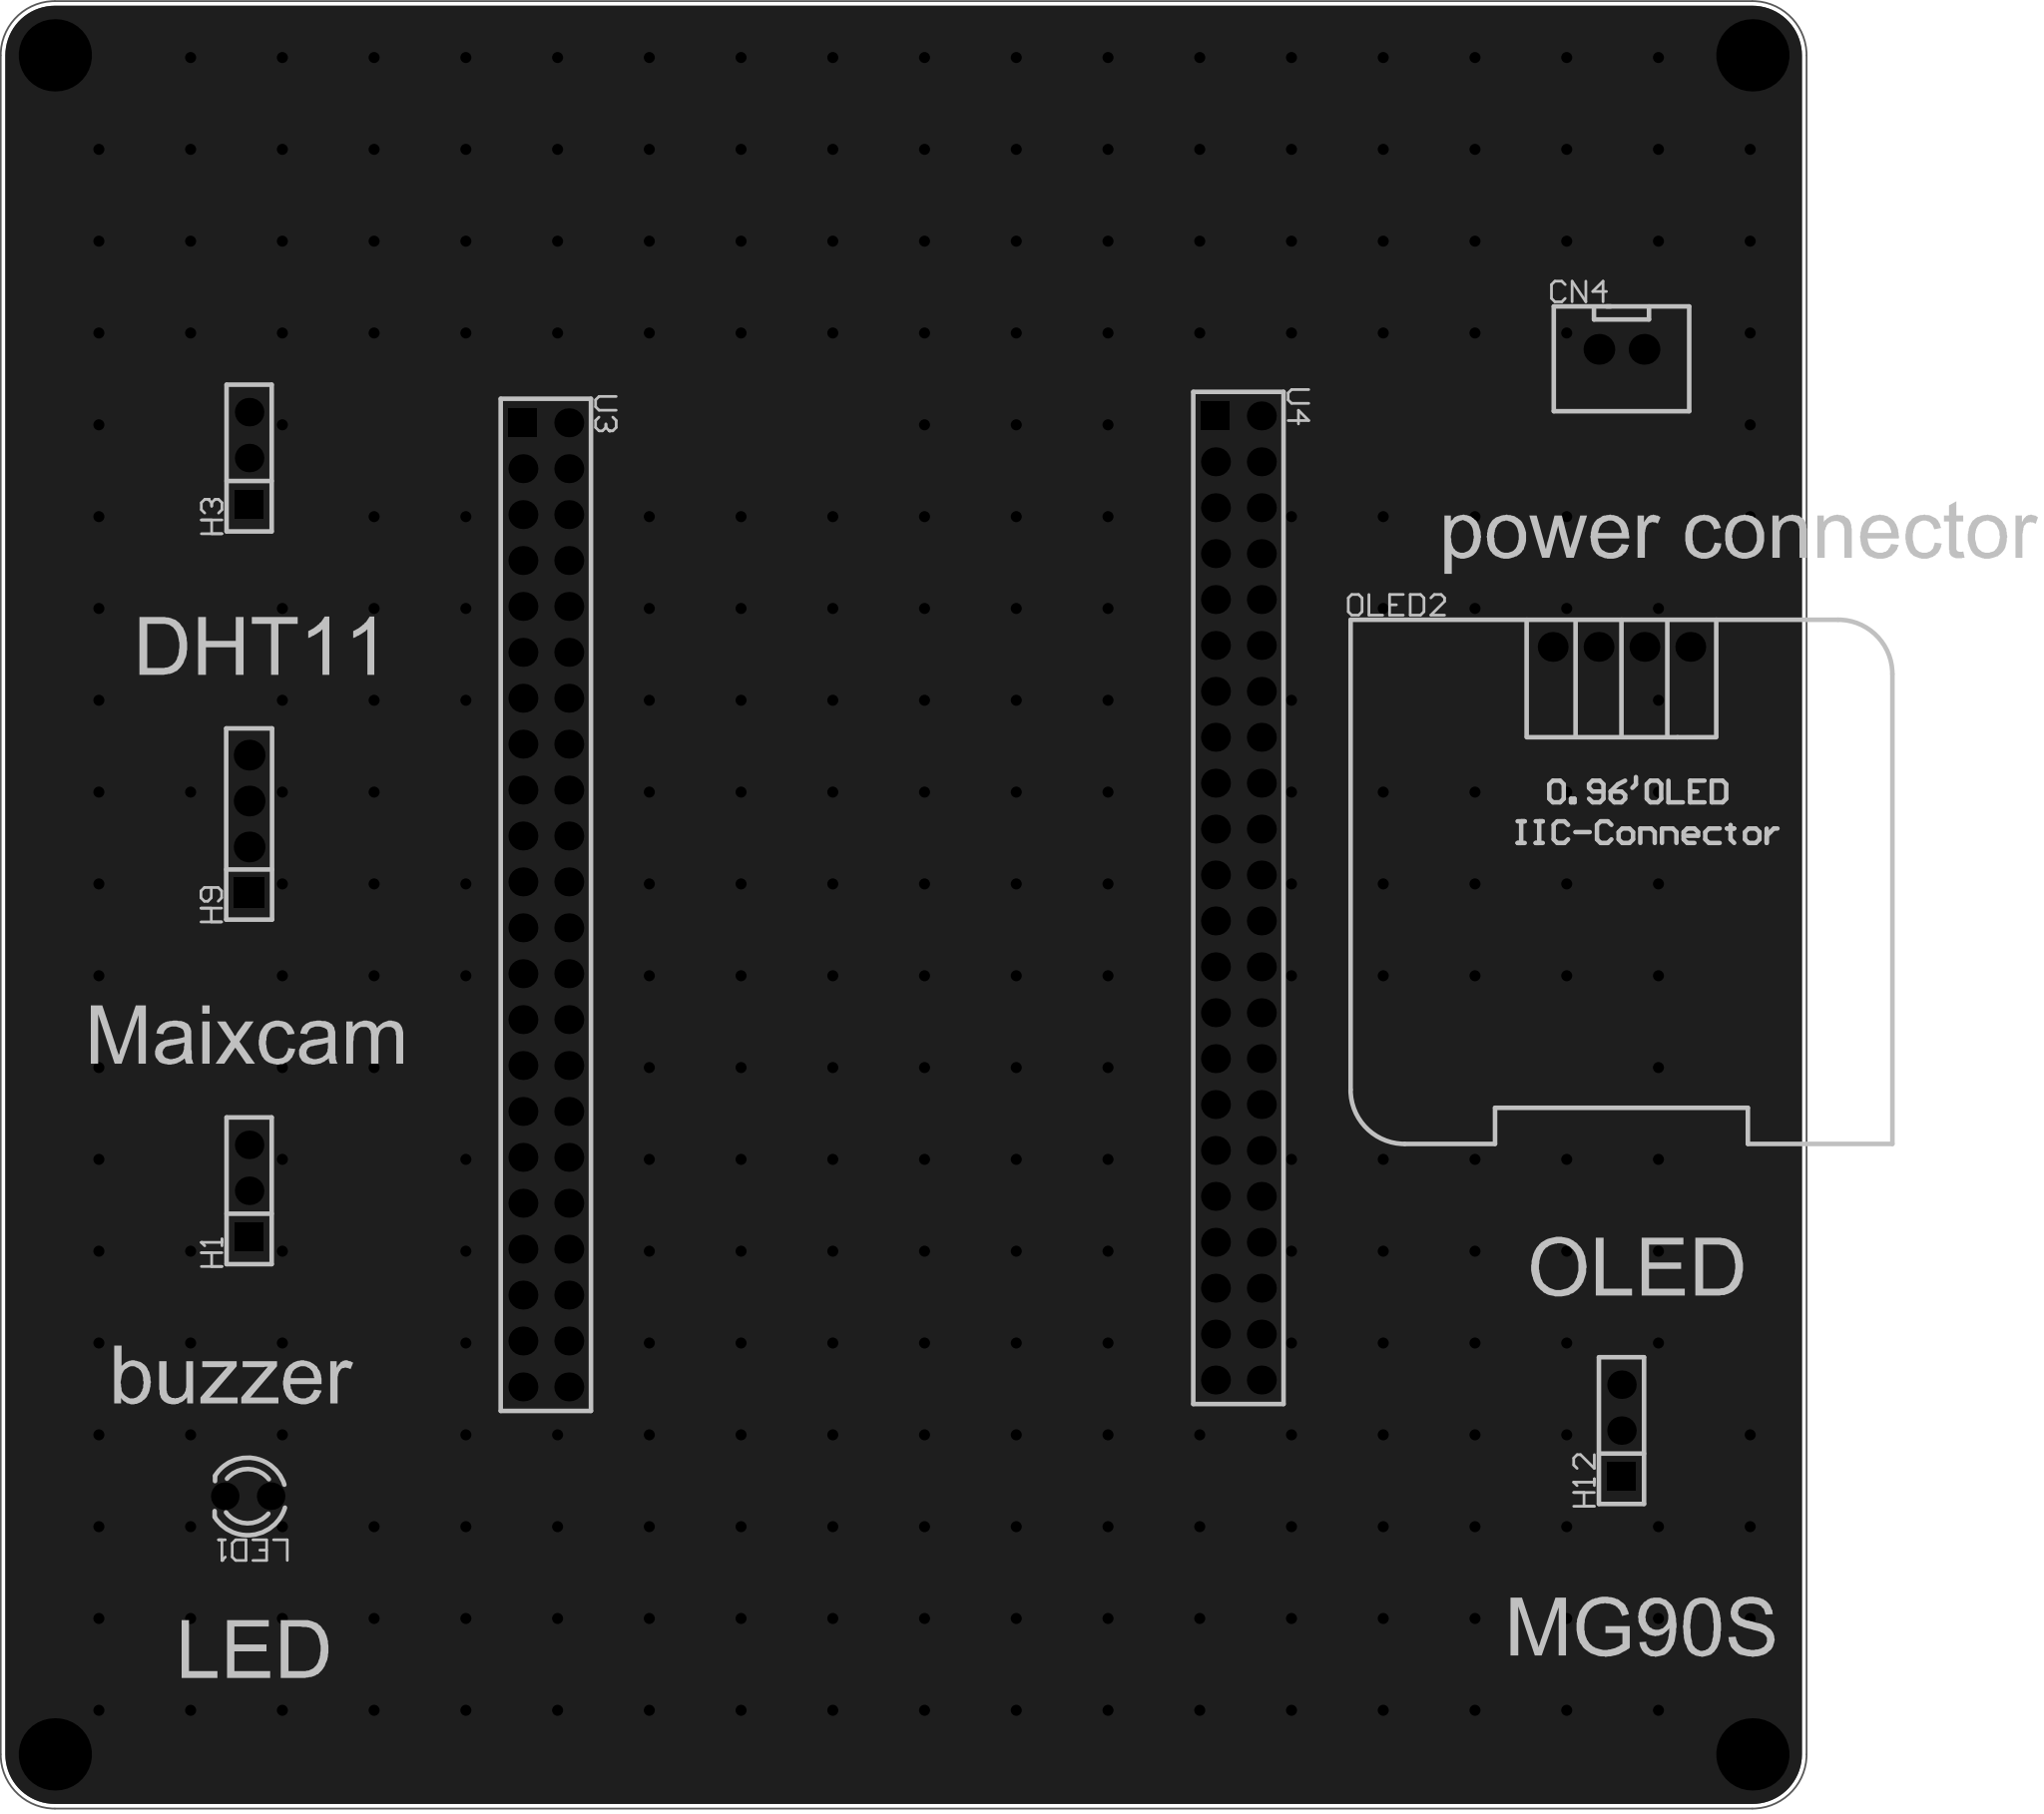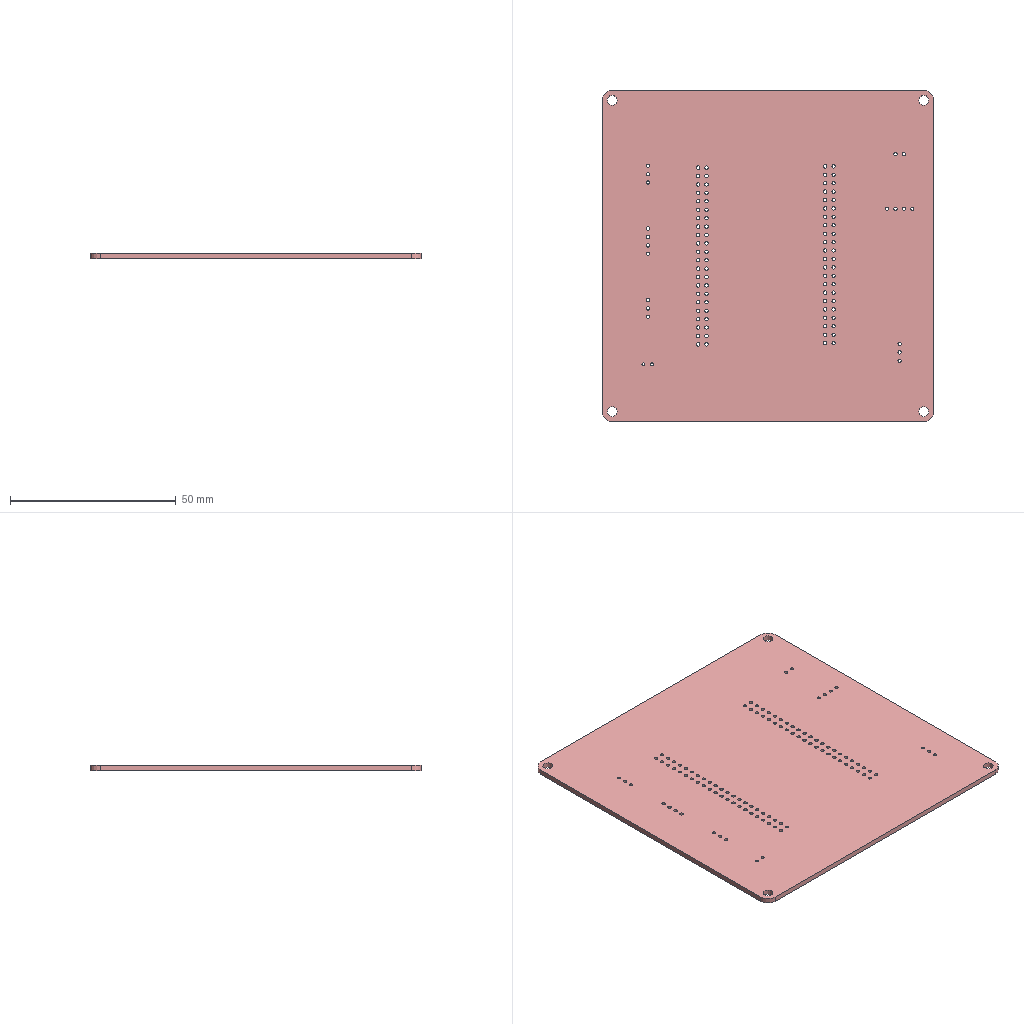Circuit board layout | Altium Designer | box 100 x 100 x 1.6 mm
Layer stack:
# Altium Designer layer stack of  (unit mm; dielectric type: 0 none, 1 core, 2 prepreg, 3 surface material)
index,name,kind,layer,copper_thickness_mm,dielectric_type,dielectric_thickness_mm,dielectric_material,dielectric_constant
0,Top Paste Mask Layer,other,,,,,,
1,Top Silkscreen Layer,other,,,,,,
2,Top Solder Mask Layer,dielectric,,,3,0.01,,3.3
3,Top Layer,copper,Top Layer,0.035,,,,
4,Dielectric1,dielectric,,,3,1.51,FR4,4.5
5,Bottom Layer,copper,Bottom Layer,0.035,,,,
6,Bottom Solder Mask Layer,dielectric,,,3,0.01,,3.3
7,Bottom Silkscreen Layer,other,,,,,,
8,Bottom Paste Mask Layer,other,,,,,,
# drill layer pairs: low layer,high layer
drill_pair,Top Layer,Bottom Layer
Part placement:
Designator,Comment,Layer,Footprint,Center-X(mm),Center-Y(mm),Rotation
CN4,XH2.54*2P_through-hole,TopLayer,CONN-TH_2P-P2.50-XH2.54-2P,181.102,161.671,0
H1,,TopLayer,HDR-TH_3P-P2.54-V-F,105.109,115.117,90
H3,,TopLayer,HDR-TH_3P-P2.54-V-F,105.109,155.656,90
H9,,TopLayer,HDR-TH_4P-P2.54-V-F,105.109,135.409,90
LED1,,TopLayer,LED_TH-3mm,105.029,98.221,180
OLED2,,TopLayer,0.96OLED_4P,181.102,145.209,0
U3,through-hole pin header_2.54_2*22,TopLayer,HDR-TH_44P-P2.54-V-M-R2-C22-S2.54,121.539,130.937,270
U4,through-hole pin header_2.54_2*22,TopLayer,HDR-TH_44P-P2.54-V-M-R2-C22-S2.54,159.889,131.318,270
H12,,TopLayer,HDR-TH_3P-P2.54-V-F,181.102,101.849,90
Pad and via stacks:
# Altium Designer via and pad stacks of  (unit mm). Each distinct definition once, with the count of objects using it.
# via: kind,start_layer,end_layer,hole_mm,diameter_mm,mode(0 simple;1 top-mid-bottom;2 full stack),diameter_per_layer,count,example_net
# pad: kind,layer,hole_mm,hole_type(0 round;1 square;2 slot),plating,top_size,top_shape(1 round;2 rect;3 octagon;9 rounded rect),mid_size,bottom_size,mode,footprint,size_per_layer,count,example
pad,Multi-Layer,3,0,plated,4x4,1,4x4,4x4,0,,,4,1
pad,Multi-Layer,1.05,0,plated,1.7x1.7,1,1.7x1.7,1.7x1.7,0,CONN-TH_2P-P2.50-XH2.54-2P,,2,CN4.2
pad,Multi-Layer,1.02,0,plated,1.575x1.575,1,1.575x1.575,1.575x1.575,0,HDR-TH_3P-P2.54-V-F,,6,H1.3
pad,Multi-Layer,1.02,0,plated,1.575x1.575,2,1.575x1.575,1.575x1.575,0,HDR-TH_3P-P2.54-V-F,,3,H1.1
pad,Multi-Layer,1.1,0,plated,1.7x1.7,2,1.7x1.7,1.7x1.7,0,HDR-TH_4P-P2.54-V-F,,1,H9.1
pad,Multi-Layer,1.1,0,plated,1.7x1.7,1,1.7x1.7,1.7x1.7,0,HDR-TH_4P-P2.54-V-F,,3,H9.2
pad,Multi-Layer,0.9144,0,plated,1.524x1.524,1,1.524x1.524,1.524x1.524,0,LED_TH-3mm,,2,LED1.1
pad,Multi-Layer,1,0,plated,1.65x1.65,1,1.65x1.65,1.65x1.65,0,0.96OLED_4P,,4,OLED2.4
pad,Multi-Layer,1.02,0,plated,1.6x1.6,1,1.6x1.6,1.6x1.6,0,HDR-TH_44P-P2.54-V-M-R2-C22-S2.54,,86,U3.44
pad,Multi-Layer,1.02,0,plated,1.6x1.6,2,1.6x1.6,1.6x1.6,0,HDR-TH_44P-P2.54-V-M-R2-C22-S2.54,,2,U3.1
via,Top Layer,Bottom Layer,0.3048,0.61,0,,291,GND
Copper pours:
name,layer,net,type(0 solid;1 hatched;2 none)
Bottom Layer-GND,Bottom Layer,GND,0
Top Layer-GND,Top Layer,GND,0
Design rules, without the lines most boards share:
# Altium Designer design rules of  (exported by Altium Designer, unit mm)
# columns: name | kind | enabled | priority | scope1 | scope2 | descriptor | typed fields (field=value)
Copper_copperRegion_copperThickness1oz | 0 | disabled | 4 | All | All | Clearance Constraint (Gap=5.984mil) (Disabled)(All),(All) | gap=0.152
Copper_copperRegion_copperThickness1oz_1 | 63 | disabled | 4 | All | All | Board Clearance Constraint (Gap=0mil) (Disabled)(All) |
Copper_copperRegion_Copper_copperRegion | 0 | disabled | 5 | All | All | Clearance Constraint (Gap=5.984mil) (Disabled)(All),(All) | gap=0.152
Copper_copperRegion_Copper_copperRegion_1 | 63 | disabled | 5 | All | All | Board Clearance Constraint (Gap=0mil) (Disabled)(All) |
copperThickness1oz | 0 | enabled | 6 | All | All | Clearance Constraint (Gap=5.984mil) (All),(All) | gap=0.152
copperThickness1oz_1 | 63 | enabled | 6 | All | All | Board Clearance Constraint (Gap=0mil) (All) |
copperRegion_copperThickness1oz | 20 | disabled | 1 | All | All | Polygon Connect Rule(Relief Connect )(Conductor Width=10mil) (Relief Angle=90 Angle) (Entries=4) (Air Gap Width=10mil) (Disabled)(All),(All) | connect_style(0=relief,1=direct,2=none)=0 relief_conductor_width=0.254 relief_entries=4
copperRegion_Copper_copperRegion | 20 | disabled | 2 | All | All | Polygon Connect Rule(Relief Connect )(Conductor Width=10mil) (Relief Angle=90 Angle) (Entries=4) (Air Gap Width=10mil) (Disabled)(All),(All) | connect_style(0=relief,1=direct,2=none)=0 relief_conductor_width=0.254 relief_entries=4
copperRegion | 20 | enabled | 3 | All | All | Polygon Connect Rule(Relief Connect )(Conductor Width=10mil) (Relief Angle=90 Angle) (Entries=4) (Air Gap Width=10mil) (All),(All) | connect_style(0=relief,1=direct,2=none)=0 relief_conductor_width=0.254 relief_entries=4